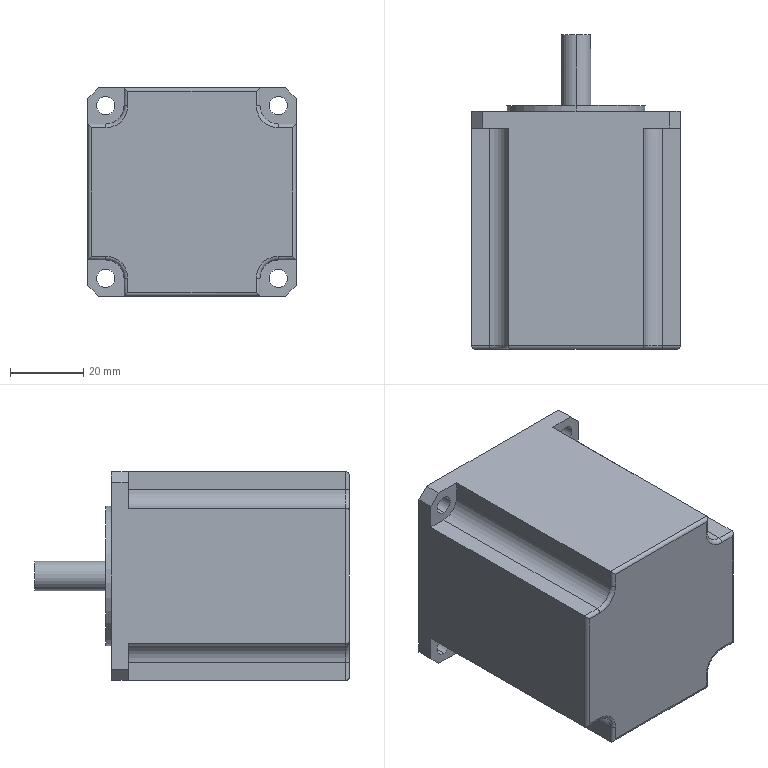Part | NX | 1 solid | 56 faces | box 57 x 86 x 57 mm | volume 190967 mm3 | cylinder 28 | plane 24 | torus 4 | commonest cylinder face diameters 2 x12 5 x8 10 x4 8 x2 38.1 x2